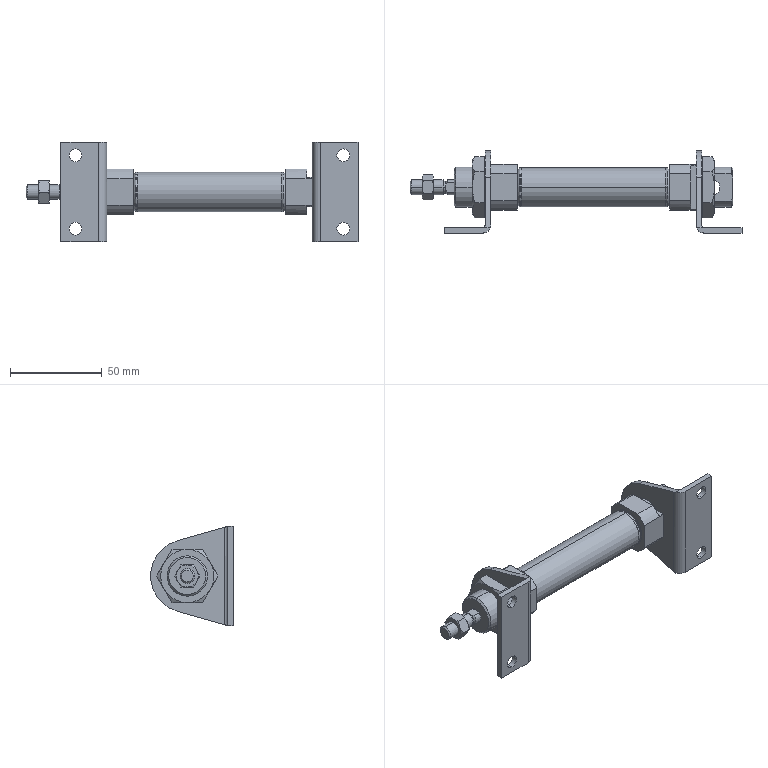Part | SolidWorks | 7 solids | 218 faces | box 181 x 45 x 54 mm | volume 67508 mm3 | plane 86 | cylinder 72 | cone 56 | torus 4 | commonest cylinder face diameters 7 x8 8 x8 22 x8 29 x8 21.4 x6 8.566 x4